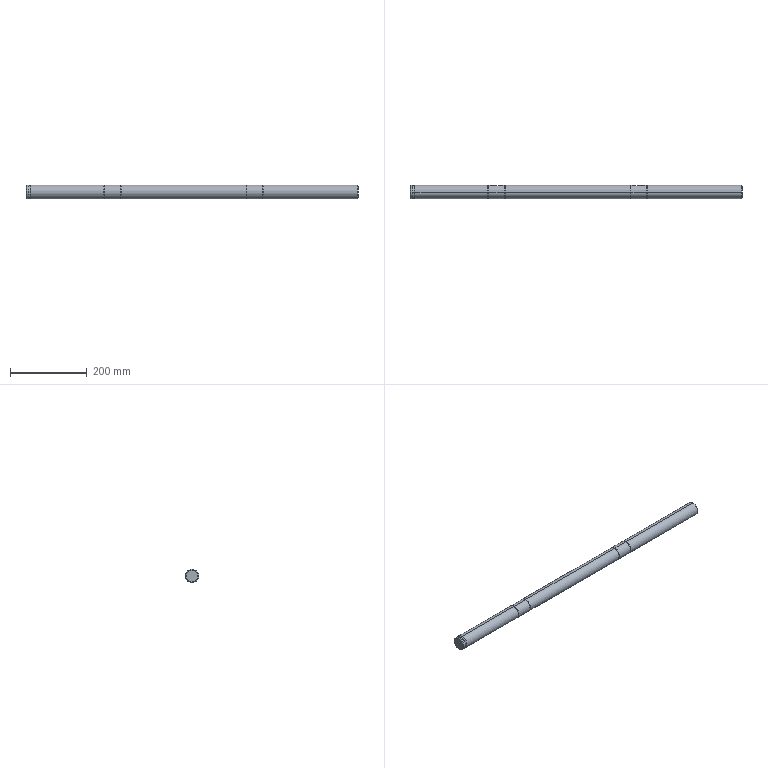Part | STEP file | IN-01-21-01 | 1 solid | 46 faces | box 865 x 35 x 35 mm | volume 828041 mm3 | cylinder 24 | plane 16 | cone 4 | spline 2 | commonest cylinder face diameters 35 x12 33 x8 10 x4